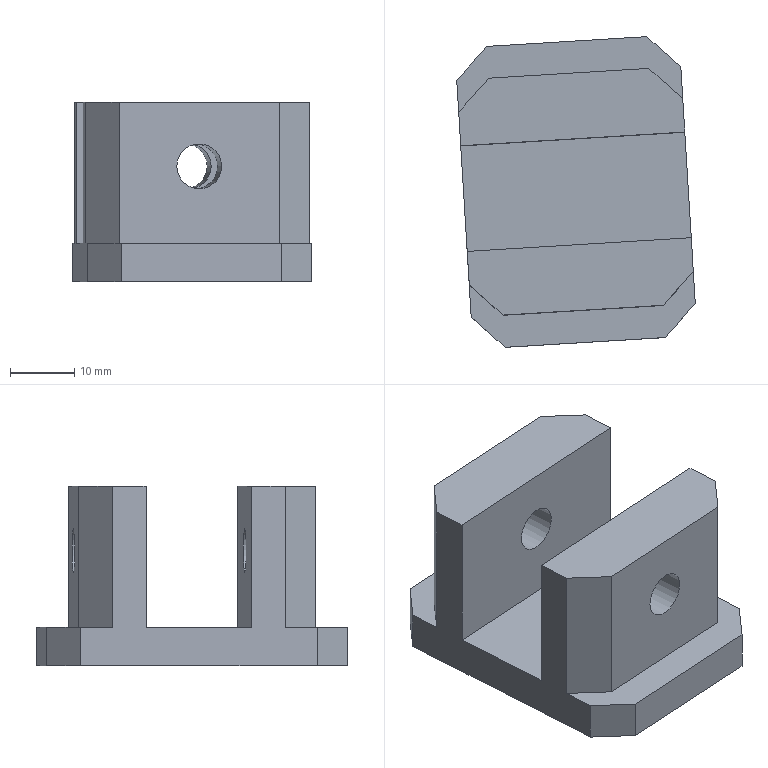Part | STEP file | 车灯-后视镜_id514_x_t | 1 solid | 24 faces | box 37.194 x 48.439 x 28 mm | volume 23466 mm3 | plane 22 | cylinder 2 | commonest cylinder face diameters 7 x2
STEP:
#1=CARTESIAN_POINT('',(104.807,-84.828,-249.5));
#2=VERTEX_POINT('',#1);
#3=CARTESIAN_POINT('',(103.8,-68.359,-249.5));
#4=VERTEX_POINT('',#3);
#5=CARTESIAN_POINT('',(105.372,-94.061,-249.5));
#6=DIRECTION('',(-0.06105,0.9981,0.));
#7=VECTOR('',#6,1.);
#8=LINE('',#5,#7);
#9=EDGE_CURVE('',#2,#4,#8,.T.);
#10=ORIENTED_EDGE('',*,*,#9,.T.);
#11=CARTESIAN_POINT('',(68.865,-70.496,-249.5));
#12=VERTEX_POINT('',#11);
#13=CARTESIAN_POINT('',(91.853,-69.09,-249.5));
#14=DIRECTION('',(0.9981,0.06105,0.));
#15=VECTOR('',#14,1.);
#16=LINE('',#13,#15);
#17=EDGE_CURVE('',#12,#4,#16,.T.);
#18=ORIENTED_EDGE('',*,*,#17,.F.);
#19=CARTESIAN_POINT('',(69.872,-86.965,-249.5));
#20=VERTEX_POINT('',#19);
#21=CARTESIAN_POINT('',(70.437,-96.198,-249.5));
#22=DIRECTION('',(0.06105,-0.9981,0.));
#23=VECTOR('',#22,1.);
#24=LINE('',#21,#23);
#25=EDGE_CURVE('',#12,#20,#24,.T.);
#26=ORIENTED_EDGE('',*,*,#25,.T.);
#27=CARTESIAN_POINT('',(92.861,-85.559,-249.5));
#28=DIRECTION('',(-0.9981,-0.06105,0.));
#29=VECTOR('',#28,1.);
#30=LINE('',#27,#29);
#31=EDGE_CURVE('',#2,#20,#30,.T.);
#32=ORIENTED_EDGE('',*,*,#31,.F.);
#33=EDGE_LOOP('',(#10,#18,#26,#32));
#34=FACE_OUTER_BOUND('',#33,.T.);
#35=CARTESIAN_POINT('',(100.188,-94.378,-249.5));
#36=DIRECTION('',(0.,0.,1.));
#37=DIRECTION('',(-0.9981,-0.06105,0.));
#38=AXIS2_PLACEMENT_3D('',#35,#36,#37);
#39=PLANE('',#38);
#40=ADVANCED_FACE('',(#34),#39,.T.);
#41=CARTESIAN_POINT('',(105.433,-95.059,-249.5));
#42=VERTEX_POINT('',#41);
#43=CARTESIAN_POINT('',(105.127,-90.068,-249.5));
#44=VERTEX_POINT('',#43);
#45=CARTESIAN_POINT('',(104.67,-82.582,-249.5));
#46=DIRECTION('',(-0.06105,0.9981,0.));
#47=VECTOR('',#46,1.);
#48=LINE('',#45,#47);
#49=EDGE_CURVE('',#42,#44,#48,.T.);
#50=ORIENTED_EDGE('',*,*,#49,.T.);
#51=CARTESIAN_POINT('',(100.442,-95.364,-249.5));
#52=VERTEX_POINT('',#51);
#53=CARTESIAN_POINT('',(105.127,-90.068,-249.5));
#54=DIRECTION('',(0.6626,0.749,0.));
#55=VECTOR('',#54,1.);
#56=LINE('',#53,#55);
#57=EDGE_CURVE('',#52,#44,#56,.T.);
#58=ORIENTED_EDGE('',*,*,#57,.F.);
#59=CARTESIAN_POINT('',(75.489,-96.89,-249.5));
#60=VERTEX_POINT('',#59);
#61=CARTESIAN_POINT('',(88.824,-96.075,-249.5));
#62=DIRECTION('',(0.9981,0.06105,0.));
#63=VECTOR('',#62,1.);
#64=LINE('',#61,#63);
#65=EDGE_CURVE('',#60,#52,#64,.T.);
#66=ORIENTED_EDGE('',*,*,#65,.F.);
#67=CARTESIAN_POINT('',(70.193,-92.205,-249.5));
#68=VERTEX_POINT('',#67);
#69=CARTESIAN_POINT('',(75.489,-96.89,-249.5));
#70=DIRECTION('',(0.749,-0.6626,0.));
#71=VECTOR('',#70,1.);
#72=LINE('',#69,#71);
#73=EDGE_CURVE('',#68,#60,#72,.T.);
#74=ORIENTED_EDGE('',*,*,#73,.F.);
#75=CARTESIAN_POINT('',(70.498,-97.196,-249.5));
#76=VERTEX_POINT('',#75);
#77=CARTESIAN_POINT('',(69.735,-84.719,-249.5));
#78=DIRECTION('',(0.06105,-0.9981,0.));
#79=VECTOR('',#78,1.);
#80=LINE('',#77,#79);
#81=EDGE_CURVE('',#68,#76,#80,.T.);
#82=ORIENTED_EDGE('',*,*,#81,.T.);
#83=CARTESIAN_POINT('',(75.794,-101.881,-249.5));
#84=VERTEX_POINT('',#83);
#85=CARTESIAN_POINT('',(75.794,-101.881,-249.5));
#86=DIRECTION('',(-0.749,0.6626,0.));
#87=VECTOR('',#86,1.);
#88=LINE('',#85,#87);
#89=EDGE_CURVE('',#84,#76,#88,.T.);
#90=ORIENTED_EDGE('',*,*,#89,.F.);
#91=CARTESIAN_POINT('',(100.747,-100.355,-249.5));
#92=VERTEX_POINT('',#91);
#93=CARTESIAN_POINT('',(100.554,-100.367,-249.5));
#94=DIRECTION('',(0.9981,0.06105,0.));
#95=VECTOR('',#94,1.);
#96=LINE('',#93,#95);
#97=EDGE_CURVE('',#84,#92,#96,.T.);
#98=ORIENTED_EDGE('',*,*,#97,.T.);
#99=CARTESIAN_POINT('',(105.433,-95.059,-249.5));
#100=DIRECTION('',(-0.6626,-0.749,0.));
#101=VECTOR('',#100,1.);
#102=LINE('',#99,#101);
#103=EDGE_CURVE('',#42,#92,#102,.T.);
#104=ORIENTED_EDGE('',*,*,#103,.F.);
#105=EDGE_LOOP('',(#50,#58,#66,#74,#82,#90,#98,#104));
#106=FACE_OUTER_BOUND('',#105,.T.);
#107=CARTESIAN_POINT('',(99.486,-82.899,-249.5));
#108=DIRECTION('',(0.,0.,1.));
#109=DIRECTION('',(-0.9981,-0.06105,0.));
#110=AXIS2_PLACEMENT_3D('',#107,#108,#109);
#111=PLANE('',#110);
#112=ADVANCED_FACE('',(#106),#111,.T.);
#113=CARTESIAN_POINT('',(97.878,-53.443,-249.5));
#114=VERTEX_POINT('',#113);
#115=CARTESIAN_POINT('',(72.925,-54.969,-249.5));
#116=VERTEX_POINT('',#115);
#117=CARTESIAN_POINT('',(97.685,-53.454,-249.5));
#118=DIRECTION('',(-0.9981,-0.06105,0.));
#119=VECTOR('',#118,1.);
#120=LINE('',#117,#119);
#121=EDGE_CURVE('',#114,#116,#120,.T.);
#122=ORIENTED_EDGE('',*,*,#121,.T.);
#123=CARTESIAN_POINT('',(68.239,-60.265,-249.5));
#124=VERTEX_POINT('',#123);
#125=CARTESIAN_POINT('',(68.239,-60.265,-249.5));
#126=DIRECTION('',(0.6626,0.749,0.));
#127=VECTOR('',#126,1.);
#128=LINE('',#125,#127);
#129=EDGE_CURVE('',#124,#116,#128,.T.);
#130=ORIENTED_EDGE('',*,*,#129,.F.);
#131=CARTESIAN_POINT('',(68.544,-65.255,-249.5));
#132=VERTEX_POINT('',#131);
#133=CARTESIAN_POINT('',(71.139,-107.676,-249.5));
#134=DIRECTION('',(0.06105,-0.9981,0.));
#135=VECTOR('',#134,1.);
#136=LINE('',#133,#135);
#137=EDGE_CURVE('',#124,#132,#136,.T.);
#138=ORIENTED_EDGE('',*,*,#137,.T.);
#139=CARTESIAN_POINT('',(73.23,-59.959,-249.5));
#140=VERTEX_POINT('',#139);
#141=CARTESIAN_POINT('',(68.544,-65.255,-249.5));
#142=DIRECTION('',(-0.6626,-0.749,0.));
#143=VECTOR('',#142,1.);
#144=LINE('',#141,#143);
#145=EDGE_CURVE('',#140,#132,#144,.T.);
#146=ORIENTED_EDGE('',*,*,#145,.F.);
#147=CARTESIAN_POINT('',(98.183,-58.433,-249.5));
#148=VERTEX_POINT('',#147);
#149=CARTESIAN_POINT('',(86.565,-59.144,-249.5));
#150=DIRECTION('',(-0.9981,-0.06105,0.));
#151=VECTOR('',#150,1.);
#152=LINE('',#149,#151);
#153=EDGE_CURVE('',#148,#140,#152,.T.);
#154=ORIENTED_EDGE('',*,*,#153,.F.);
#155=CARTESIAN_POINT('',(103.479,-63.119,-249.5));
#156=VERTEX_POINT('',#155);
#157=CARTESIAN_POINT('',(98.183,-58.433,-249.5));
#158=DIRECTION('',(-0.749,0.6626,0.));
#159=VECTOR('',#158,1.);
#160=LINE('',#157,#159);
#161=EDGE_CURVE('',#156,#148,#160,.T.);
#162=ORIENTED_EDGE('',*,*,#161,.F.);
#163=CARTESIAN_POINT('',(103.174,-58.128,-249.5));
#164=VERTEX_POINT('',#163);
#165=CARTESIAN_POINT('',(106.074,-105.539,-249.5));
#166=DIRECTION('',(-0.06105,0.9981,0.));
#167=VECTOR('',#166,1.);
#168=LINE('',#165,#167);
#169=EDGE_CURVE('',#156,#164,#168,.T.);
#170=ORIENTED_EDGE('',*,*,#169,.T.);
#171=CARTESIAN_POINT('',(97.878,-53.443,-249.5));
#172=DIRECTION('',(0.749,-0.6626,0.));
#173=VECTOR('',#172,1.);
#174=LINE('',#171,#173);
#175=EDGE_CURVE('',#114,#164,#174,.T.);
#176=ORIENTED_EDGE('',*,*,#175,.F.);
#177=EDGE_LOOP('',(#122,#130,#138,#146,#154,#162,#170,#176));
#178=FACE_OUTER_BOUND('',#177,.T.);
#179=CARTESIAN_POINT('',(100.89,-105.856,-249.5));
#180=DIRECTION('',(0.,0.,1.));
#181=DIRECTION('',(-0.9981,-0.06105,0.));
#182=AXIS2_PLACEMENT_3D('',#179,#180,#181);
#183=PLANE('',#182);
#184=ADVANCED_FACE('',(#178),#183,.T.);
#185=ORIENTED_EDGE('',*,*,#97,.F.);
#186=CARTESIAN_POINT('',(75.794,-101.881,-255.5));
#187=VERTEX_POINT('',#186);
#188=CARTESIAN_POINT('',(75.794,-101.881,-255.5));
#189=DIRECTION('',(0.,0.,1.));
#190=VECTOR('',#189,1.);
#191=LINE('',#188,#190);
#192=EDGE_CURVE('',#187,#84,#191,.T.);
#193=ORIENTED_EDGE('',*,*,#192,.F.);
#194=CARTESIAN_POINT('',(100.747,-100.355,-255.5));
#195=VERTEX_POINT('',#194);
#196=CARTESIAN_POINT('',(89.129,-101.066,-255.5));
#197=DIRECTION('',(-0.9981,-0.06105,0.));
#198=VECTOR('',#197,1.);
#199=LINE('',#196,#198);
#200=EDGE_CURVE('',#195,#187,#199,.T.);
#201=ORIENTED_EDGE('',*,*,#200,.F.);
#202=CARTESIAN_POINT('',(100.747,-100.355,-255.5));
#203=DIRECTION('',(0.,0.,-1.));
#204=VECTOR('',#203,1.);
#205=LINE('',#202,#204);
#206=EDGE_CURVE('',#92,#195,#205,.T.);
#207=ORIENTED_EDGE('',*,*,#206,.F.);
#208=EDGE_LOOP('',(#185,#193,#201,#207));
#209=FACE_OUTER_BOUND('',#208,.T.);
#210=CARTESIAN_POINT('',(89.129,-101.066,-255.5));
#211=DIRECTION('',(0.06105,-0.9981,0.));
#212=DIRECTION('',(0.,0.,-1.));
#213=AXIS2_PLACEMENT_3D('',#210,#211,#212);
#214=PLANE('',#213);
#215=ADVANCED_FACE('',(#209),#214,.T.);
#216=CARTESIAN_POINT('',(103.174,-58.128,-255.5));
#217=VERTEX_POINT('',#216);
#218=CARTESIAN_POINT('',(105.433,-95.059,-255.5));
#219=VERTEX_POINT('',#218);
#220=CARTESIAN_POINT('',(103.54,-64.117,-255.5));
#221=DIRECTION('',(0.06105,-0.9981,0.));
#222=VECTOR('',#221,1.);
#223=LINE('',#220,#222);
#224=EDGE_CURVE('',#217,#219,#223,.T.);
#225=ORIENTED_EDGE('',*,*,#224,.F.);
#226=CARTESIAN_POINT('',(103.174,-58.128,-255.5));
#227=DIRECTION('',(0.,0.,-1.));
#228=VECTOR('',#227,1.);
#229=LINE('',#226,#228);
#230=EDGE_CURVE('',#164,#217,#229,.T.);
#231=ORIENTED_EDGE('',*,*,#230,.F.);
#232=ORIENTED_EDGE('',*,*,#169,.F.);
#233=CARTESIAN_POINT('',(103.479,-63.119,-227.5));
#234=VERTEX_POINT('',#233);
#235=CARTESIAN_POINT('',(103.479,-63.119,-255.5));
#236=DIRECTION('',(0.,0.,-1.));
#237=VECTOR('',#236,1.);
#238=LINE('',#235,#237);
#239=EDGE_CURVE('',#234,#156,#238,.T.);
#240=ORIENTED_EDGE('',*,*,#239,.F.);
#241=CARTESIAN_POINT('',(103.8,-68.359,-227.5));
#242=VERTEX_POINT('',#241);
#243=CARTESIAN_POINT('',(103.815,-68.608,-227.5));
#244=DIRECTION('',(-0.06105,0.9981,0.));
#245=VECTOR('',#244,1.);
#246=LINE('',#243,#245);
#247=EDGE_CURVE('',#242,#234,#246,.T.);
#248=ORIENTED_EDGE('',*,*,#247,.F.);
#249=CARTESIAN_POINT('',(103.8,-68.359,-255.5));
#250=DIRECTION('',(0.,0.,-1.));
#251=VECTOR('',#250,1.);
#252=LINE('',#249,#251);
#253=EDGE_CURVE('',#242,#4,#252,.T.);
#254=ORIENTED_EDGE('',*,*,#253,.T.);
#255=ORIENTED_EDGE('',*,*,#9,.F.);
#256=CARTESIAN_POINT('',(104.807,-84.828,-227.5));
#257=VERTEX_POINT('',#256);
#258=CARTESIAN_POINT('',(104.807,-84.828,-243.));
#259=DIRECTION('',(0.,0.,-1.));
#260=VECTOR('',#259,1.);
#261=LINE('',#258,#260);
#262=EDGE_CURVE('',#257,#2,#261,.T.);
#263=ORIENTED_EDGE('',*,*,#262,.F.);
#264=CARTESIAN_POINT('',(105.127,-90.068,-227.5));
#265=VERTEX_POINT('',#264);
#266=CARTESIAN_POINT('',(103.265,-59.625,-227.5));
#267=DIRECTION('',(-0.06105,0.9981,0.));
#268=VECTOR('',#267,1.);
#269=LINE('',#266,#268);
#270=EDGE_CURVE('',#265,#257,#269,.T.);
#271=ORIENTED_EDGE('',*,*,#270,.F.);
#272=CARTESIAN_POINT('',(105.127,-90.068,-255.5));
#273=DIRECTION('',(0.,0.,1.));
#274=VECTOR('',#273,1.);
#275=LINE('',#272,#274);
#276=EDGE_CURVE('',#44,#265,#275,.T.);
#277=ORIENTED_EDGE('',*,*,#276,.F.);
#278=ORIENTED_EDGE('',*,*,#49,.F.);
#279=CARTESIAN_POINT('',(105.433,-95.059,-255.5));
#280=DIRECTION('',(0.,0.,1.));
#281=VECTOR('',#280,1.);
#282=LINE('',#279,#281);
#283=EDGE_CURVE('',#219,#42,#282,.T.);
#284=ORIENTED_EDGE('',*,*,#283,.F.);
#285=EDGE_LOOP('',(#225,#231,#232,#240,#248,#254,#255,#263,#271,#277,#278,#284));
#286=FACE_OUTER_BOUND('',#285,.T.);
#287=CARTESIAN_POINT('',(103.54,-64.117,-255.5));
#288=DIRECTION('',(0.9981,0.06105,0.));
#289=DIRECTION('',(0.,0.,1.));
#290=AXIS2_PLACEMENT_3D('',#287,#288,#289);
#291=PLANE('',#290);
#292=ADVANCED_FACE('',(#286),#291,.T.);
#293=CARTESIAN_POINT('',(72.925,-54.969,-255.5));
#294=VERTEX_POINT('',#293);
#295=CARTESIAN_POINT('',(97.878,-53.443,-255.5));
#296=VERTEX_POINT('',#295);
#297=CARTESIAN_POINT('',(86.26,-54.153,-255.5));
#298=DIRECTION('',(0.9981,0.06105,0.));
#299=VECTOR('',#298,1.);
#300=LINE('',#297,#299);
#301=EDGE_CURVE('',#294,#296,#300,.T.);
#302=ORIENTED_EDGE('',*,*,#301,.F.);
#303=CARTESIAN_POINT('',(72.925,-54.969,-255.5));
#304=DIRECTION('',(0.,0.,-1.));
#305=VECTOR('',#304,1.);
#306=LINE('',#303,#305);
#307=EDGE_CURVE('',#116,#294,#306,.T.);
#308=ORIENTED_EDGE('',*,*,#307,.F.);
#309=ORIENTED_EDGE('',*,*,#121,.F.);
#310=CARTESIAN_POINT('',(97.878,-53.443,-255.5));
#311=DIRECTION('',(0.,0.,1.));
#312=VECTOR('',#311,1.);
#313=LINE('',#310,#312);
#314=EDGE_CURVE('',#296,#114,#313,.T.);
#315=ORIENTED_EDGE('',*,*,#314,.F.);
#316=EDGE_LOOP('',(#302,#308,#309,#315));
#317=FACE_OUTER_BOUND('',#316,.T.);
#318=CARTESIAN_POINT('',(86.26,-54.153,-255.5));
#319=DIRECTION('',(-0.06105,0.9981,0.));
#320=DIRECTION('',(0.,0.,1.));
#321=AXIS2_PLACEMENT_3D('',#318,#319,#320);
#322=PLANE('',#321);
#323=ADVANCED_FACE('',(#317),#322,.T.);
#324=ORIENTED_EDGE('',*,*,#81,.F.);
#325=CARTESIAN_POINT('',(70.193,-92.205,-227.5));
#326=VERTEX_POINT('',#325);
#327=CARTESIAN_POINT('',(70.193,-92.205,-255.5));
#328=DIRECTION('',(0.,0.,-1.));
#329=VECTOR('',#328,1.);
#330=LINE('',#327,#329);
#331=EDGE_CURVE('',#326,#68,#330,.T.);
#332=ORIENTED_EDGE('',*,*,#331,.F.);
#333=CARTESIAN_POINT('',(69.872,-86.965,-227.5));
#334=VERTEX_POINT('',#333);
#335=CARTESIAN_POINT('',(68.331,-61.762,-227.5));
#336=DIRECTION('',(0.06105,-0.9981,0.));
#337=VECTOR('',#336,1.);
#338=LINE('',#335,#337);
#339=EDGE_CURVE('',#334,#326,#338,.T.);
#340=ORIENTED_EDGE('',*,*,#339,.F.);
#341=CARTESIAN_POINT('',(69.872,-86.965,-243.));
#342=DIRECTION('',(0.,0.,1.));
#343=VECTOR('',#342,1.);
#344=LINE('',#341,#343);
#345=EDGE_CURVE('',#20,#334,#344,.T.);
#346=ORIENTED_EDGE('',*,*,#345,.F.);
#347=ORIENTED_EDGE('',*,*,#25,.F.);
#348=CARTESIAN_POINT('',(68.865,-70.496,-227.5));
#349=VERTEX_POINT('',#348);
#350=CARTESIAN_POINT('',(68.865,-70.496,-255.5));
#351=DIRECTION('',(0.,0.,1.));
#352=VECTOR('',#351,1.);
#353=LINE('',#350,#352);
#354=EDGE_CURVE('',#12,#349,#353,.T.);
#355=ORIENTED_EDGE('',*,*,#354,.T.);
#356=CARTESIAN_POINT('',(68.544,-65.255,-227.5));
#357=VERTEX_POINT('',#356);
#358=CARTESIAN_POINT('',(68.88,-70.745,-227.5));
#359=DIRECTION('',(0.06105,-0.9981,0.));
#360=VECTOR('',#359,1.);
#361=LINE('',#358,#360);
#362=EDGE_CURVE('',#357,#349,#361,.T.);
#363=ORIENTED_EDGE('',*,*,#362,.F.);
#364=CARTESIAN_POINT('',(68.544,-65.255,-255.5));
#365=DIRECTION('',(0.,0.,1.));
#366=VECTOR('',#365,1.);
#367=LINE('',#364,#366);
#368=EDGE_CURVE('',#132,#357,#367,.T.);
#369=ORIENTED_EDGE('',*,*,#368,.F.);
#370=ORIENTED_EDGE('',*,*,#137,.F.);
#371=CARTESIAN_POINT('',(68.239,-60.265,-255.5));
#372=VERTEX_POINT('',#371);
#373=CARTESIAN_POINT('',(68.239,-60.265,-255.5));
#374=DIRECTION('',(0.,0.,1.));
#375=VECTOR('',#374,1.);
#376=LINE('',#373,#375);
#377=EDGE_CURVE('',#372,#124,#376,.T.);
#378=ORIENTED_EDGE('',*,*,#377,.F.);
#379=CARTESIAN_POINT('',(70.498,-97.196,-255.5));
#380=VERTEX_POINT('',#379);
#381=CARTESIAN_POINT('',(68.605,-66.254,-255.5));
#382=DIRECTION('',(-0.06105,0.9981,0.));
#383=VECTOR('',#382,1.);
#384=LINE('',#381,#383);
#385=EDGE_CURVE('',#380,#372,#384,.T.);
#386=ORIENTED_EDGE('',*,*,#385,.F.);
#387=CARTESIAN_POINT('',(70.498,-97.196,-255.5));
#388=DIRECTION('',(0.,0.,-1.));
#389=VECTOR('',#388,1.);
#390=LINE('',#387,#389);
#391=EDGE_CURVE('',#76,#380,#390,.T.);
#392=ORIENTED_EDGE('',*,*,#391,.F.);
#393=EDGE_LOOP('',(#324,#332,#340,#346,#347,#355,#363,#369,#370,#378,#386,#392));
#394=FACE_OUTER_BOUND('',#393,.T.);
#395=CARTESIAN_POINT('',(68.605,-66.254,-255.5));
#396=DIRECTION('',(-0.9981,-0.06105,0.));
#397=DIRECTION('',(0.,0.,-1.));
#398=AXIS2_PLACEMENT_3D('',#395,#396,#397);
#399=PLANE('',#398);
#400=ADVANCED_FACE('',(#394),#399,.T.);
#401=ORIENTED_EDGE('',*,*,#200,.T.);
#402=CARTESIAN_POINT('',(75.794,-101.881,-255.5));
#403=DIRECTION('',(0.749,-0.6626,0.));
#404=VECTOR('',#403,1.);
#405=LINE('',#402,#404);
#406=EDGE_CURVE('',#380,#187,#405,.T.);
#407=ORIENTED_EDGE('',*,*,#406,.F.);
#408=ORIENTED_EDGE('',*,*,#385,.T.);
#409=CARTESIAN_POINT('',(68.239,-60.265,-255.5));
#410=DIRECTION('',(-0.6626,-0.749,0.));
#411=VECTOR('',#410,1.);
#412=LINE('',#409,#411);
#413=EDGE_CURVE('',#294,#372,#412,.T.);
#414=ORIENTED_EDGE('',*,*,#413,.F.);
#415=ORIENTED_EDGE('',*,*,#301,.T.);
#416=CARTESIAN_POINT('',(97.878,-53.443,-255.5));
#417=DIRECTION('',(-0.749,0.6626,0.));
#418=VECTOR('',#417,1.);
#419=LINE('',#416,#418);
#420=EDGE_CURVE('',#217,#296,#419,.T.);
#421=ORIENTED_EDGE('',*,*,#420,.F.);
#422=ORIENTED_EDGE('',*,*,#224,.T.);
#423=CARTESIAN_POINT('',(105.433,-95.059,-255.5));
#424=DIRECTION('',(0.6626,0.749,0.));
#425=VECTOR('',#424,1.);
#426=LINE('',#423,#425);
#427=EDGE_CURVE('',#195,#219,#426,.T.);
#428=ORIENTED_EDGE('',*,*,#427,.F.);
#429=EDGE_LOOP('',(#401,#407,#408,#414,#415,#421,#422,#428));
#430=FACE_OUTER_BOUND('',#429,.T.);
#431=CARTESIAN_POINT('',(86.931,-65.133,-255.5));
#432=DIRECTION('',(0.,0.,-1.));
#433=DIRECTION('',(0.9981,0.06105,0.));
#434=AXIS2_PLACEMENT_3D('',#431,#432,#433);
#435=PLANE('',#434);
#436=ADVANCED_FACE('',(#430),#435,.T.);
#437=CARTESIAN_POINT('',(82.213,-59.41,-237.501));
#438=VERTEX_POINT('',#437);
#439=CARTESIAN_POINT('',(85.706,-59.196,-237.501));
#440=DIRECTION('',(0.06105,-0.9981,0.));
#441=DIRECTION('',(-0.9981,-0.06105,0.));
#442=AXIS2_PLACEMENT_3D('',#439,#440,#441);
#443=CIRCLE('',#442,3.5);
#444=EDGE_CURVE('',#438,#438,#443,.T.);
#445=ORIENTED_EDGE('',*,*,#444,.T.);
#446=EDGE_LOOP('',(#445));
#447=FACE_BOUND('',#446,.T.);
#448=ORIENTED_EDGE('',*,*,#153,.T.);
#449=CARTESIAN_POINT('',(73.23,-59.959,-227.5));
#450=VERTEX_POINT('',#449);
#451=CARTESIAN_POINT('',(73.23,-59.959,-255.5));
#452=DIRECTION('',(0.,0.,-1.));
#453=VECTOR('',#452,1.);
#454=LINE('',#451,#453);
#455=EDGE_CURVE('',#450,#140,#454,.T.);
#456=ORIENTED_EDGE('',*,*,#455,.F.);
#457=CARTESIAN_POINT('',(98.183,-58.433,-227.5));
#458=VERTEX_POINT('',#457);
#459=CARTESIAN_POINT('',(86.565,-59.144,-227.5));
#460=DIRECTION('',(-0.9981,-0.06105,0.));
#461=VECTOR('',#460,1.);
#462=LINE('',#459,#461);
#463=EDGE_CURVE('',#458,#450,#462,.T.);
#464=ORIENTED_EDGE('',*,*,#463,.F.);
#465=CARTESIAN_POINT('',(98.183,-58.433,-255.5));
#466=DIRECTION('',(0.,0.,1.));
#467=VECTOR('',#466,1.);
#468=LINE('',#465,#467);
#469=EDGE_CURVE('',#148,#458,#468,.T.);
#470=ORIENTED_EDGE('',*,*,#469,.F.);
#471=EDGE_LOOP('',(#448,#456,#464,#470));
#472=FACE_BOUND('',#471,.T.);
#473=CARTESIAN_POINT('',(86.565,-59.144,-255.5));
#474=DIRECTION('',(-0.06105,0.9981,0.));
#475=DIRECTION('',(0.,0.,1.));
#476=AXIS2_PLACEMENT_3D('',#473,#474,#475);
#477=PLANE('',#476);
#478=ADVANCED_FACE('',(#447,#472),#477,.T.);
#479=CARTESIAN_POINT('',(82.839,-69.641,-237.501));
#480=VERTEX_POINT('',#479);
#481=CARTESIAN_POINT('',(86.332,-69.427,-237.501));
#482=DIRECTION('',(0.06105,-0.9981,0.));
#483=DIRECTION('',(-0.9981,-0.06105,0.));
#484=AXIS2_PLACEMENT_3D('',#481,#482,#483);
#485=CIRCLE('',#484,3.5);
#486=EDGE_CURVE('',#480,#480,#485,.T.);
#487=ORIENTED_EDGE('',*,*,#486,.F.);
#488=EDGE_LOOP('',(#487));
#489=FACE_BOUND('',#488,.T.);
#490=CARTESIAN_POINT('',(87.191,-69.375,-227.5));
#491=DIRECTION('',(0.9981,0.06105,0.));
#492=VECTOR('',#491,1.);
#493=LINE('',#490,#492);
#494=EDGE_CURVE('',#349,#242,#493,.T.);
#495=ORIENTED_EDGE('',*,*,#494,.F.);
#496=ORIENTED_EDGE('',*,*,#354,.F.);
#497=ORIENTED_EDGE('',*,*,#17,.T.);
#498=ORIENTED_EDGE('',*,*,#253,.F.);
#499=EDGE_LOOP('',(#495,#496,#497,#498));
#500=FACE_BOUND('',#499,.T.);
#501=CARTESIAN_POINT('',(91.853,-69.09,-243.));
#502=DIRECTION('',(-0.06105,0.9981,0.));
#503=DIRECTION('',(0.,0.,1.));
#504=AXIS2_PLACEMENT_3D('',#501,#502,#503);
#505=PLANE('',#504);
#506=ADVANCED_FACE('',(#489,#500),#505,.F.);
#507=ORIENTED_EDGE('',*,*,#463,.T.);
#508=CARTESIAN_POINT('',(68.544,-65.255,-227.5));
#509=DIRECTION('',(0.6626,0.749,0.));
#510=VECTOR('',#509,1.);
#511=LINE('',#508,#510);
#512=EDGE_CURVE('',#357,#450,#511,.T.);
#513=ORIENTED_EDGE('',*,*,#512,.F.);
#514=ORIENTED_EDGE('',*,*,#362,.T.);
#515=ORIENTED_EDGE('',*,*,#494,.T.);
#516=ORIENTED_EDGE('',*,*,#247,.T.);
#517=CARTESIAN_POINT('',(98.183,-58.433,-227.5));
#518=DIRECTION('',(0.749,-0.6626,0.));
#519=VECTOR('',#518,1.);
#520=LINE('',#517,#519);
#521=EDGE_CURVE('',#458,#234,#520,.T.);
#522=ORIENTED_EDGE('',*,*,#521,.F.);
#523=EDGE_LOOP('',(#507,#513,#514,#515,#516,#522));
#524=FACE_OUTER_BOUND('',#523,.T.);
#525=CARTESIAN_POINT('',(87.206,-69.624,-227.5));
#526=DIRECTION('',(0.,0.,1.));
#527=DIRECTION('',(-0.9981,-0.06105,0.));
#528=AXIS2_PLACEMENT_3D('',#525,#526,#527);
#529=PLANE('',#528);
#530=ADVANCED_FACE('',(#524),#529,.T.);
#531=CARTESIAN_POINT('',(75.489,-96.89,-227.5));
#532=VERTEX_POINT('',#531);
#533=CARTESIAN_POINT('',(100.442,-95.364,-227.5));
#534=VERTEX_POINT('',#533);
#535=CARTESIAN_POINT('',(88.824,-96.075,-227.5));
#536=DIRECTION('',(0.9981,0.06105,0.));
#537=VECTOR('',#536,1.);
#538=LINE('',#535,#537);
#539=EDGE_CURVE('',#532,#534,#538,.T.);
#540=ORIENTED_EDGE('',*,*,#539,.T.);
#541=CARTESIAN_POINT('',(105.127,-90.068,-227.5));
#542=DIRECTION('',(-0.6626,-0.749,0.));
#543=VECTOR('',#542,1.);
#544=LINE('',#541,#543);
#545=EDGE_CURVE('',#265,#534,#544,.T.);
#546=ORIENTED_EDGE('',*,*,#545,.F.);
#547=ORIENTED_EDGE('',*,*,#270,.T.);
#548=CARTESIAN_POINT('',(92.861,-85.559,-227.5));
#549=DIRECTION('',(0.9981,0.06105,0.));
#550=VECTOR('',#549,1.);
#551=LINE('',#548,#550);
#552=EDGE_CURVE('',#334,#257,#551,.T.);
#553=ORIENTED_EDGE('',*,*,#552,.F.);
#554=ORIENTED_EDGE('',*,*,#339,.T.);
#555=CARTESIAN_POINT('',(75.489,-96.89,-227.5));
#556=DIRECTION('',(-0.749,0.6626,0.));
#557=VECTOR('',#556,1.);
#558=LINE('',#555,#557);
#559=EDGE_CURVE('',#532,#326,#558,.T.);
#560=ORIENTED_EDGE('',*,*,#559,.F.);
#561=EDGE_LOOP('',(#540,#546,#547,#553,#554,#560));
#562=FACE_OUTER_BOUND('',#561,.T.);
#563=CARTESIAN_POINT('',(86.656,-60.641,-227.5));
#564=DIRECTION('',(0.,0.,1.));
#565=DIRECTION('',(-0.9981,-0.06105,0.));
#566=AXIS2_PLACEMENT_3D('',#563,#564,#565);
#567=PLANE('',#566);
#568=ADVANCED_FACE('',(#562),#567,.T.);
#569=CARTESIAN_POINT('',(91.459,-95.914,-237.501));
#570=VERTEX_POINT('',#569);
#571=CARTESIAN_POINT('',(87.965,-96.127,-237.501));
#572=DIRECTION('',(-0.06105,0.9981,0.));
#573=DIRECTION('',(0.9981,0.06105,0.));
#574=AXIS2_PLACEMENT_3D('',#571,#572,#573);
#575=CIRCLE('',#574,3.5);
#576=EDGE_CURVE('',#570,#570,#575,.T.);
#577=ORIENTED_EDGE('',*,*,#576,.T.);
#578=EDGE_LOOP('',(#577));
#579=FACE_BOUND('',#578,.T.);
#580=ORIENTED_EDGE('',*,*,#65,.T.);
#581=CARTESIAN_POINT('',(100.442,-95.364,-255.5));
#582=DIRECTION('',(0.,0.,-1.));
#583=VECTOR('',#582,1.);
#584=LINE('',#581,#583);
#585=EDGE_CURVE('',#534,#52,#584,.T.);
#586=ORIENTED_EDGE('',*,*,#585,.F.);
#587=ORIENTED_EDGE('',*,*,#539,.F.);
#588=CARTESIAN_POINT('',(75.489,-96.89,-255.5));
#589=DIRECTION('',(0.,0.,1.));
#590=VECTOR('',#589,1.);
#591=LINE('',#588,#590);
#592=EDGE_CURVE('',#60,#532,#591,.T.);
#593=ORIENTED_EDGE('',*,*,#592,.F.);
#594=EDGE_LOOP('',(#580,#586,#587,#593));
#595=FACE_BOUND('',#594,.T.);
#596=CARTESIAN_POINT('',(88.824,-96.075,-255.5));
#597=DIRECTION('',(0.06105,-0.9981,0.));
#598=DIRECTION('',(0.,0.,-1.));
#599=AXIS2_PLACEMENT_3D('',#596,#597,#598);
#600=PLANE('',#599);
#601=ADVANCED_FACE('',(#579,#595),#600,.T.);
#602=CARTESIAN_POINT('',(90.833,-85.683,-237.501));
#603=VERTEX_POINT('',#602);
#604=CARTESIAN_POINT('',(87.34,-85.896,-237.501));
#605=DIRECTION('',(-0.06105,0.9981,0.));
#606=DIRECTION('',(0.9981,0.06105,0.));
#607=AXIS2_PLACEMENT_3D('',#604,#605,#606);
#608=CIRCLE('',#607,3.5);
#609=EDGE_CURVE('',#603,#603,#608,.T.);
#610=ORIENTED_EDGE('',*,*,#609,.F.);
#611=EDGE_LOOP('',(#610));
#612=FACE_BOUND('',#611,.T.);
#613=ORIENTED_EDGE('',*,*,#262,.T.);
#614=ORIENTED_EDGE('',*,*,#31,.T.);
#615=ORIENTED_EDGE('',*,*,#345,.T.);
#616=ORIENTED_EDGE('',*,*,#552,.T.);
#617=EDGE_LOOP('',(#613,#614,#615,#616));
#618=FACE_BOUND('',#617,.T.);
#619=CARTESIAN_POINT('',(92.861,-85.559,-243.));
#620=DIRECTION('',(0.06105,-0.9981,0.));
#621=DIRECTION('',(0.,0.,-1.));
#622=AXIS2_PLACEMENT_3D('',#619,#620,#621);
#623=PLANE('',#622);
#624=ADVANCED_FACE('',(#612,#618),#623,.F.);
#625=ORIENTED_EDGE('',*,*,#576,.F.);
#626=EDGE_LOOP('',(#625));
#627=FACE_BOUND('',#626,.T.);
#628=ORIENTED_EDGE('',*,*,#609,.T.);
#629=EDGE_LOOP('',(#628));
#630=FACE_BOUND('',#629,.T.);
#631=CARTESIAN_POINT('',(89.272,-117.49,-237.501));
#632=DIRECTION('',(-0.06105,0.9981,0.));
#633=DIRECTION('',(0.,0.,1.));
#634=AXIS2_PLACEMENT_3D('',#631,#632,#633);
#635=CYLINDRICAL_SURFACE('',#634,3.5);
#636=ADVANCED_FACE('',(#627,#630),#635,.F.);
#637=ORIENTED_EDGE('',*,*,#444,.F.);
#638=EDGE_LOOP('',(#637));
#639=FACE_BOUND('',#638,.T.);
#640=ORIENTED_EDGE('',*,*,#486,.T.);
#641=EDGE_LOOP('',(#640));
#642=FACE_BOUND('',#641,.T.);
#643=CARTESIAN_POINT('',(89.821,-126.473,-237.501));
#644=DIRECTION('',(-0.06105,0.9981,0.));
#645=DIRECTION('',(0.,0.,1.));
#646=AXIS2_PLACEMENT_3D('',#643,#644,#645);
#647=CYLINDRICAL_SURFACE('',#646,3.5);
#648=ADVANCED_FACE('',(#639,#642),#647,.F.);
#649=ORIENTED_EDGE('',*,*,#161,.T.);
#650=ORIENTED_EDGE('',*,*,#469,.T.);
#651=ORIENTED_EDGE('',*,*,#521,.T.);
#652=ORIENTED_EDGE('',*,*,#239,.T.);
#653=EDGE_LOOP('',(#649,#650,#651,#652));
#654=FACE_OUTER_BOUND('',#653,.T.);
#655=CARTESIAN_POINT('',(98.183,-58.433,-255.5));
#656=DIRECTION('',(-0.6626,-0.749,0.));
#657=DIRECTION('',(-0.749,0.6626,0.));
#658=AXIS2_PLACEMENT_3D('',#655,#656,#657);
#659=PLANE('',#658);
#660=ADVANCED_FACE('',(#654),#659,.F.);
#661=ORIENTED_EDGE('',*,*,#145,.T.);
#662=ORIENTED_EDGE('',*,*,#368,.T.);
#663=ORIENTED_EDGE('',*,*,#512,.T.);
#664=ORIENTED_EDGE('',*,*,#455,.T.);
#665=EDGE_LOOP('',(#661,#662,#663,#664));
#666=FACE_OUTER_BOUND('',#665,.T.);
#667=CARTESIAN_POINT('',(68.544,-65.255,-255.5));
#668=DIRECTION('',(0.749,-0.6626,0.));
#669=DIRECTION('',(-0.6626,-0.749,0.));
#670=AXIS2_PLACEMENT_3D('',#667,#668,#669);
#671=PLANE('',#670);
#672=ADVANCED_FACE('',(#666),#671,.F.);
#673=ORIENTED_EDGE('',*,*,#73,.T.);
#674=ORIENTED_EDGE('',*,*,#592,.T.);
#675=ORIENTED_EDGE('',*,*,#559,.T.);
#676=ORIENTED_EDGE('',*,*,#331,.T.);
#677=EDGE_LOOP('',(#673,#674,#675,#676));
#678=FACE_OUTER_BOUND('',#677,.T.);
#679=CARTESIAN_POINT('',(75.489,-96.89,-255.5));
#680=DIRECTION('',(0.6626,0.749,0.));
#681=DIRECTION('',(0.749,-0.6626,0.));
#682=AXIS2_PLACEMENT_3D('',#679,#680,#681);
#683=PLANE('',#682);
#684=ADVANCED_FACE('',(#678),#683,.F.);
#685=ORIENTED_EDGE('',*,*,#57,.T.);
#686=ORIENTED_EDGE('',*,*,#276,.T.);
#687=ORIENTED_EDGE('',*,*,#545,.T.);
#688=ORIENTED_EDGE('',*,*,#585,.T.);
#689=EDGE_LOOP('',(#685,#686,#687,#688));
#690=FACE_OUTER_BOUND('',#689,.T.);
#691=CARTESIAN_POINT('',(105.127,-90.068,-255.5));
#692=DIRECTION('',(-0.749,0.6626,0.));
#693=DIRECTION('',(0.6626,0.749,0.));
#694=AXIS2_PLACEMENT_3D('',#691,#692,#693);
#695=PLANE('',#694);
#696=ADVANCED_FACE('',(#690),#695,.F.);
#697=ORIENTED_EDGE('',*,*,#427,.T.);
#698=ORIENTED_EDGE('',*,*,#283,.T.);
#699=ORIENTED_EDGE('',*,*,#103,.T.);
#700=ORIENTED_EDGE('',*,*,#206,.T.);
#701=EDGE_LOOP('',(#697,#698,#699,#700));
#702=FACE_OUTER_BOUND('',#701,.T.);
#703=CARTESIAN_POINT('',(105.433,-95.059,-255.5));
#704=DIRECTION('',(-0.749,0.6626,0.));
#705=DIRECTION('',(0.6626,0.749,0.));
#706=AXIS2_PLACEMENT_3D('',#703,#704,#705);
#707=PLANE('',#706);
#708=ADVANCED_FACE('',(#702),#707,.F.);
#709=ORIENTED_EDGE('',*,*,#406,.T.);
#710=ORIENTED_EDGE('',*,*,#192,.T.);
#711=ORIENTED_EDGE('',*,*,#89,.T.);
#712=ORIENTED_EDGE('',*,*,#391,.T.);
#713=EDGE_LOOP('',(#709,#710,#711,#712));
#714=FACE_OUTER_BOUND('',#713,.T.);
#715=CARTESIAN_POINT('',(75.794,-101.881,-255.5));
#716=DIRECTION('',(0.6626,0.749,0.));
#717=DIRECTION('',(0.749,-0.6626,0.));
#718=AXIS2_PLACEMENT_3D('',#715,#716,#717);
#719=PLANE('',#718);
#720=ADVANCED_FACE('',(#714),#719,.F.);
#721=ORIENTED_EDGE('',*,*,#420,.T.);
#722=ORIENTED_EDGE('',*,*,#314,.T.);
#723=ORIENTED_EDGE('',*,*,#175,.T.);
#724=ORIENTED_EDGE('',*,*,#230,.T.);
#725=EDGE_LOOP('',(#721,#722,#723,#724));
#726=FACE_OUTER_BOUND('',#725,.T.);
#727=CARTESIAN_POINT('',(97.878,-53.443,-255.5));
#728=DIRECTION('',(-0.6626,-0.749,0.));
#729=DIRECTION('',(-0.749,0.6626,0.));
#730=AXIS2_PLACEMENT_3D('',#727,#728,#729);
#731=PLANE('',#730);
#732=ADVANCED_FACE('',(#726),#731,.F.);
#733=ORIENTED_EDGE('',*,*,#413,.T.);
#734=ORIENTED_EDGE('',*,*,#377,.T.);
#735=ORIENTED_EDGE('',*,*,#129,.T.);
#736=ORIENTED_EDGE('',*,*,#307,.T.);
#737=EDGE_LOOP('',(#733,#734,#735,#736));
#738=FACE_OUTER_BOUND('',#737,.T.);
#739=CARTESIAN_POINT('',(68.239,-60.265,-255.5));
#740=DIRECTION('',(0.749,-0.6626,0.));
#741=DIRECTION('',(-0.6626,-0.749,0.));
#742=AXIS2_PLACEMENT_3D('',#739,#740,#741);
#743=PLANE('',#742);
#744=ADVANCED_FACE('',(#738),#743,.F.);
#745=CLOSED_SHELL('',(#40,#112,#184,#215,#292,#323,#400,#436,#478,#506,#530,#568,#601,#624,#636,#648,#660,#672,#684,#696,#708,#720,#732,#744));
#746=MANIFOLD_SOLID_BREP('',#745);
#747=(LENGTH_UNIT()NAMED_UNIT(*)SI_UNIT(.MILLI.,.METRE.));
#748=UNCERTAINTY_MEASURE_WITH_UNIT(LENGTH_MEASURE(0.00002),#747,'','');
#749=(NAMED_UNIT(*)PLANE_ANGLE_UNIT()SI_UNIT($,.RADIAN.));
#750=PLANE_ANGLE_MEASURE_WITH_UNIT(PLANE_ANGLE_MEASURE(0.01745),#749);
#751=DIMENSIONAL_EXPONENTS(0.,0.,0.,0.,0.,0.,0.);
#752=(CONVERSION_BASED_UNIT('DEGREE',#750)NAMED_UNIT(#751)PLANE_ANGLE_UNIT());
#753=(NAMED_UNIT(*)SI_UNIT($,.STERADIAN.)SOLID_ANGLE_UNIT());
#754=(GEOMETRIC_REPRESENTATION_CONTEXT(3)GLOBAL_UNCERTAINTY_ASSIGNED_CONTEXT((#748))GLOBAL_UNIT_ASSIGNED_CONTEXT((#747,#752,#753))REPRESENTATION_CONTEXT('',''));
#755=ADVANCED_BREP_SHAPE_REPRESENTATION('',(#746),#754);